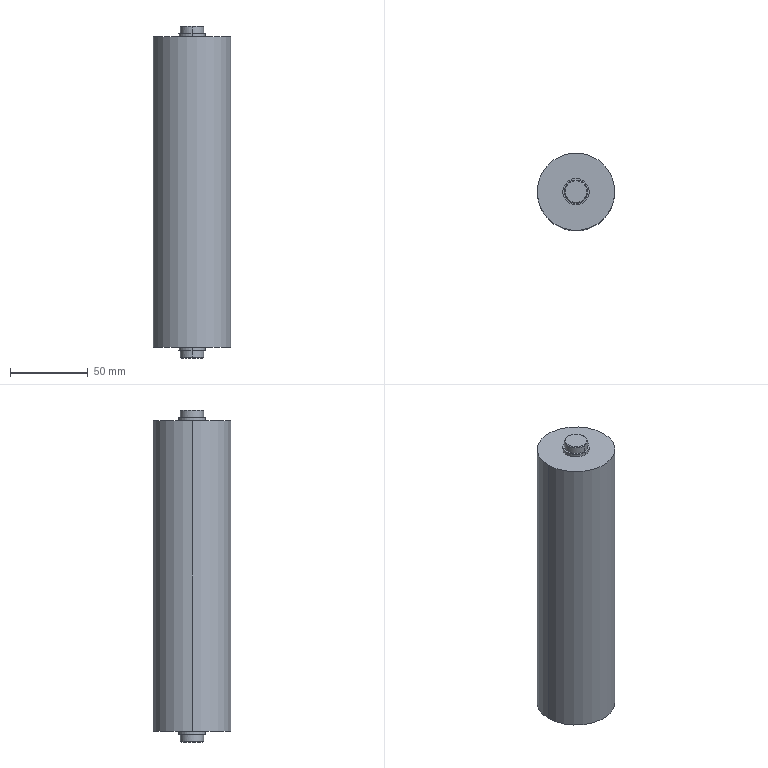Part | STEP file | 02-02 Driven mixing drum | 2 solids | 24 faces | box 50 x 50 x 214 mm | volume 578580 mm3 | cylinder 12 | plane 8 | cone 4 | commonest cylinder face diameters 15 x4 17 x4 36 x2 50 x2